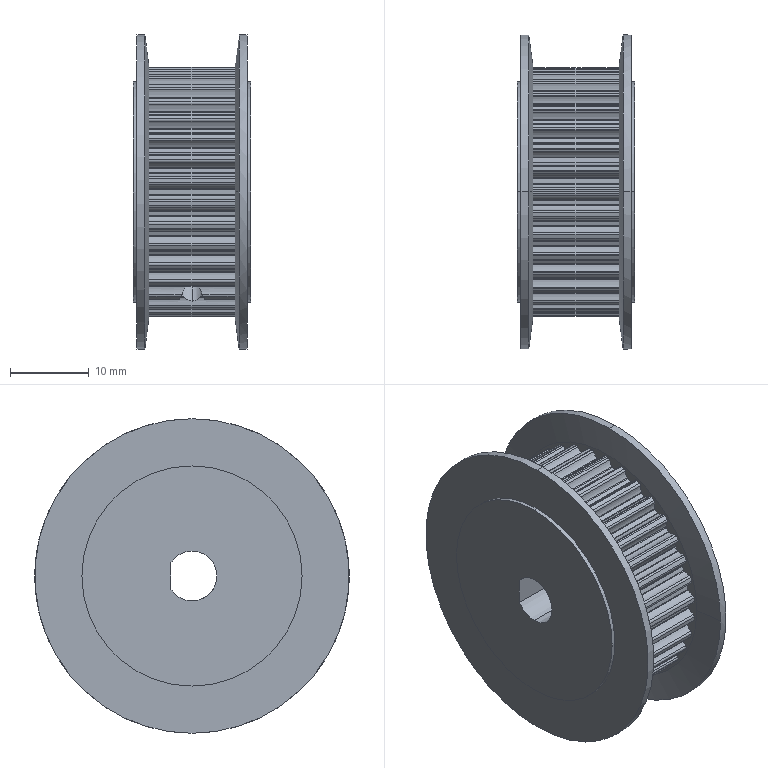Part | SolidWorks | features BaseBody 1 | 1 solid | 344 faces | box 15 x 40 x 40 mm | volume 11573 mm3 | cylinder 333 | plane 7 | cone 4 | commonest cylinder face diameters 0.56 x86 0.3 x82 3.95 x78 29.49 x36 31.71 x36 3.242 x4